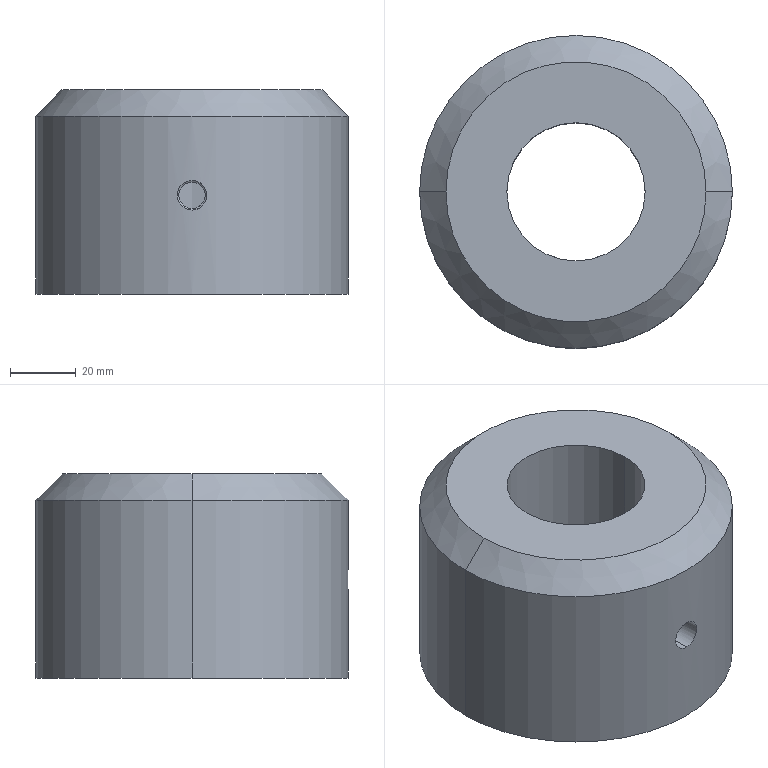Part | SolidWorks | features Chamfer 1, Extrusion 1, HoleWzd 1, ICE 1 | 1 solid | 14 faces | box 95 x 95 x 62 mm | volume 343089 mm3 | cylinder 8 | cone 4 | plane 2 | commonest cylinder face diameters 8 x2 9 x2 42 x2 95 x2
STEP:
#1=CARTESIAN_POINT('',(0.,-37.5,34.5));
#2=VERTEX_POINT('',#1);
#3=CARTESIAN_POINT('',(0.,-37.5,25.5));
#4=VERTEX_POINT('',#3);
#5=CARTESIAN_POINT('',(0.,-37.5,30.));
#6=DIRECTION('',(0.,-1.,0.));
#7=DIRECTION('',(0.,0.,-1.));
#8=AXIS2_PLACEMENT_3D('',#5,#6,#7);
#9=CIRCLE('',#8,4.5);
#10=EDGE_CURVE('',#2,#4,#9,.T.);
#11=ORIENTED_EDGE('',*,*,#10,.F.);
#12=CARTESIAN_POINT('',(0.,-47.5,34.5));
#13=VERTEX_POINT('',#12);
#14=CARTESIAN_POINT('',(0.,-47.5,34.5));
#15=DIRECTION('',(0.,-1.,0.));
#16=VECTOR('',#15,1000.);
#17=LINE('',#14,#16);
#18=EDGE_CURVE('',#2,#13,#17,.T.);
#19=ORIENTED_EDGE('',*,*,#18,.T.);
#20=CARTESIAN_POINT('',(0.,-47.5,25.5));
#21=VERTEX_POINT('',#20);
#22=CARTESIAN_POINT('',(0.,-47.5,25.5));
#23=CARTESIAN_POINT('',(-0.2975,-47.5,25.5));
#24=CARTESIAN_POINT('',(-0.59,-47.497,25.529));
#25=CARTESIAN_POINT('',(-1.165,-47.487,25.644));
#26=CARTESIAN_POINT('',(-1.451,-47.479,25.73));
#27=CARTESIAN_POINT('',(-1.996,-47.459,25.956));
#28=CARTESIAN_POINT('',(-2.255,-47.447,26.094));
#29=CARTESIAN_POINT('',(-2.744,-47.421,26.421));
#30=CARTESIAN_POINT('',(-2.975,-47.407,26.611));
#31=CARTESIAN_POINT('',(-3.39,-47.379,27.026));
#32=CARTESIAN_POINT('',(-3.576,-47.365,27.253));
#33=CARTESIAN_POINT('',(-3.905,-47.339,27.745));
#34=CARTESIAN_POINT('',(-4.045,-47.328,28.006));
#35=CARTESIAN_POINT('',(-4.269,-47.308,28.548));
#36=CARTESIAN_POINT('',(-4.356,-47.3,28.832));
#37=CARTESIAN_POINT('',(-4.471,-47.289,29.413));
#38=CARTESIAN_POINT('',(-4.5,-47.286,29.705));
#39=CARTESIAN_POINT('',(-4.5,-47.286,30.292));
#40=CARTESIAN_POINT('',(-4.471,-47.289,30.59));
#41=CARTESIAN_POINT('',(-4.356,-47.3,31.168));
#42=CARTESIAN_POINT('',(-4.271,-47.308,31.448));
#43=CARTESIAN_POINT('',(-4.045,-47.328,31.993));
#44=CARTESIAN_POINT('',(-3.904,-47.34,32.257));
#45=CARTESIAN_POINT('',(-3.579,-47.365,32.744));
#46=CARTESIAN_POINT('',(-3.393,-47.379,32.971));
#47=CARTESIAN_POINT('',(-2.972,-47.407,33.392));
#48=CARTESIAN_POINT('',(-2.745,-47.421,33.578));
#49=CARTESIAN_POINT('',(-2.258,-47.447,33.904));
#50=CARTESIAN_POINT('',(-1.995,-47.459,34.044));
#51=CARTESIAN_POINT('',(-1.45,-47.479,34.27));
#52=CARTESIAN_POINT('',(-1.169,-47.486,34.355));
#53=CARTESIAN_POINT('',(-0.5922,-47.497,34.471));
#54=CARTESIAN_POINT('',(-0.2938,-47.5,34.5));
#55=CARTESIAN_POINT('',(0.,-47.5,34.5));
#56=B_SPLINE_CURVE_WITH_KNOTS('',3,(#22,#23,#24,#25,#26,#27,#28,#29,#30,#31,#32,#33,#34,#35,#36,#37,#38,#39,#40,#41,#42,#43,#44,#45,#46,#47,#48,#49,#50,#51,#52,#53,#54,#55),.UNSPECIFIED.,.F.,.F.,(4,2,2,2,2,2,2,2,2,2,2,2,2,2,2,2,4),(0.,0.0008798,0.00176,0.002639,0.003519,0.004399,0.005279,0.006159,0.007038,0.007918,0.008798,0.009678,0.01056,0.01144,0.01232,0.0132,0.01408),.UNSPECIFIED.);
#57=EDGE_CURVE('',#21,#13,#56,.T.);
#58=ORIENTED_EDGE('',*,*,#57,.F.);
#59=CARTESIAN_POINT('',(0.,-47.5,25.5));
#60=DIRECTION('',(0.,-1.,0.));
#61=VECTOR('',#60,1000.);
#62=LINE('',#59,#61);
#63=EDGE_CURVE('',#4,#21,#62,.T.);
#64=ORIENTED_EDGE('',*,*,#63,.F.);
#65=EDGE_LOOP('',(#11,#19,#58,#64));
#66=FACE_OUTER_BOUND('',#65,.T.);
#67=CARTESIAN_POINT('',(0.,-47.5,30.));
#68=DIRECTION('',(0.,-1.,0.));
#69=DIRECTION('',(0.,0.,-1.));
#70=AXIS2_PLACEMENT_3D('',#67,#68,#69);
#71=CYLINDRICAL_SURFACE('',#70,4.5);
#72=ADVANCED_FACE('',(#66),#71,.F.);
#73=CARTESIAN_POINT('',(0.,-37.2,34.));
#74=VERTEX_POINT('',#73);
#75=CARTESIAN_POINT('',(0.,-37.2,26.));
#76=VERTEX_POINT('',#75);
#77=CARTESIAN_POINT('',(0.,-37.2,30.));
#78=DIRECTION('',(0.,-1.,0.));
#79=DIRECTION('',(0.,0.,-1.));
#80=AXIS2_PLACEMENT_3D('',#77,#78,#79);
#81=CIRCLE('',#80,4.);
#82=EDGE_CURVE('',#74,#76,#81,.T.);
#83=ORIENTED_EDGE('',*,*,#82,.F.);
#84=CARTESIAN_POINT('',(0.,-37.5,34.5));
#85=DIRECTION('',(0.,-0.515,0.8572));
#86=VECTOR('',#85,1000.);
#87=LINE('',#84,#86);
#88=EDGE_CURVE('',#74,#2,#87,.T.);
#89=ORIENTED_EDGE('',*,*,#88,.T.);
#90=ORIENTED_EDGE('',*,*,#10,.T.);
#91=CARTESIAN_POINT('',(0.,-37.5,25.5));
#92=DIRECTION('',(0.,-0.515,-0.8572));
#93=VECTOR('',#92,1000.);
#94=LINE('',#91,#93);
#95=EDGE_CURVE('',#76,#4,#94,.T.);
#96=ORIENTED_EDGE('',*,*,#95,.F.);
#97=EDGE_LOOP('',(#83,#89,#90,#96));
#98=FACE_OUTER_BOUND('',#97,.T.);
#99=CARTESIAN_POINT('',(0.,-37.5,30.));
#100=DIRECTION('',(0.,-1.,0.));
#101=DIRECTION('',(0.,0.,-1.));
#102=AXIS2_PLACEMENT_3D('',#99,#100,#101);
#103=CONICAL_SURFACE('',#102,4.5,1.03);
#104=ADVANCED_FACE('',(#98),#103,.F.);
#105=ORIENTED_EDGE('',*,*,#82,.T.);
#106=CARTESIAN_POINT('',(0.,-21.,26.));
#107=VERTEX_POINT('',#106);
#108=CARTESIAN_POINT('',(0.,-47.5,26.));
#109=DIRECTION('',(0.,1.,0.));
#110=VECTOR('',#109,1000.);
#111=LINE('',#108,#110);
#112=EDGE_CURVE('',#76,#107,#111,.T.);
#113=ORIENTED_EDGE('',*,*,#112,.T.);
#114=CARTESIAN_POINT('',(0.,-21.,34.));
#115=VERTEX_POINT('',#114);
#116=CARTESIAN_POINT('',(0.,-21.,26.));
#117=CARTESIAN_POINT('',(-0.2613,-21.,26.));
#118=CARTESIAN_POINT('',(-0.5215,-20.995,26.025));
#119=CARTESIAN_POINT('',(-1.039,-20.976,26.128));
#120=CARTESIAN_POINT('',(-1.291,-20.962,26.205));
#121=CARTESIAN_POINT('',(-1.772,-20.926,26.405));
#122=CARTESIAN_POINT('',(-2.006,-20.905,26.529));
#123=CARTESIAN_POINT('',(-2.441,-20.859,26.821));
#124=CARTESIAN_POINT('',(-2.642,-20.834,26.986));
#125=CARTESIAN_POINT('',(-3.011,-20.784,27.354));
#126=CARTESIAN_POINT('',(-3.18,-20.758,27.559));
#127=CARTESIAN_POINT('',(-3.47,-20.712,27.993));
#128=CARTESIAN_POINT('',(-3.593,-20.691,28.222));
#129=CARTESIAN_POINT('',(-3.794,-20.655,28.707));
#130=CARTESIAN_POINT('',(-3.871,-20.64,28.96));
#131=CARTESIAN_POINT('',(-3.974,-20.621,29.472));
#132=CARTESIAN_POINT('',(-4.,-20.616,29.734));
#133=CARTESIAN_POINT('',(-4.,-20.616,30.262));
#134=CARTESIAN_POINT('',(-3.974,-20.621,30.522));
#135=CARTESIAN_POINT('',(-3.873,-20.64,31.035));
#136=CARTESIAN_POINT('',(-3.795,-20.654,31.29));
#137=CARTESIAN_POINT('',(-3.595,-20.69,31.773));
#138=CARTESIAN_POINT('',(-3.473,-20.711,32.003));
#139=CARTESIAN_POINT('',(-3.182,-20.758,32.438));
#140=CARTESIAN_POINT('',(-3.014,-20.783,32.643));
#141=CARTESIAN_POINT('',(-2.647,-20.833,33.011));
#142=CARTESIAN_POINT('',(-2.446,-20.858,33.176));
#143=CARTESIAN_POINT('',(-2.007,-20.905,33.47));
#144=CARTESIAN_POINT('',(-1.777,-20.926,33.593));
#145=CARTESIAN_POINT('',(-1.296,-20.961,33.793));
#146=CARTESIAN_POINT('',(-1.043,-20.976,33.871));
#147=CARTESIAN_POINT('',(-0.5264,-20.995,33.974));
#148=CARTESIAN_POINT('',(-0.2649,-21.,34.));
#149=CARTESIAN_POINT('',(0.,-21.,34.));
#150=B_SPLINE_CURVE_WITH_KNOTS('',3,(#116,#117,#118,#119,#120,#121,#122,#123,#124,#125,#126,#127,#128,#129,#130,#131,#132,#133,#134,#135,#136,#137,#138,#139,#140,#141,#142,#143,#144,#145,#146,#147,#148,#149),.UNSPECIFIED.,.F.,.F.,(4,2,2,2,2,2,2,2,2,2,2,2,2,2,2,2,4),(0.01253,0.01332,0.0141,0.01488,0.01567,0.01645,0.01723,0.01802,0.0188,0.01958,0.02037,0.02115,0.02193,0.02272,0.0235,0.02428,0.02507),.UNSPECIFIED.);
#151=EDGE_CURVE('',#107,#115,#150,.T.);
#152=ORIENTED_EDGE('',*,*,#151,.T.);
#153=CARTESIAN_POINT('',(0.,-47.5,34.));
#154=DIRECTION('',(0.,1.,0.));
#155=VECTOR('',#154,1000.);
#156=LINE('',#153,#155);
#157=EDGE_CURVE('',#74,#115,#156,.T.);
#158=ORIENTED_EDGE('',*,*,#157,.F.);
#159=EDGE_LOOP('',(#105,#113,#152,#158));
#160=FACE_OUTER_BOUND('',#159,.T.);
#161=CARTESIAN_POINT('',(0.,-47.5,30.));
#162=DIRECTION('',(0.,1.,0.));
#163=DIRECTION('',(0.,0.,1.));
#164=AXIS2_PLACEMENT_3D('',#161,#162,#163);
#165=CYLINDRICAL_SURFACE('',#164,4.);
#166=ADVANCED_FACE('',(#160),#165,.F.);
#167=CARTESIAN_POINT('',(39.5,0.,62.));
#168=VERTEX_POINT('',#167);
#169=CARTESIAN_POINT('',(-39.5,0.,62.));
#170=VERTEX_POINT('',#169);
#171=CARTESIAN_POINT('',(0.,0.,62.));
#172=DIRECTION('',(0.,0.,1.));
#173=DIRECTION('',(1.,0.,0.));
#174=AXIS2_PLACEMENT_3D('',#171,#172,#173);
#175=CIRCLE('',#174,39.5);
#176=EDGE_CURVE('',#168,#170,#175,.T.);
#177=ORIENTED_EDGE('',*,*,#176,.F.);
#178=CARTESIAN_POINT('',(47.5,0.,54.));
#179=VERTEX_POINT('',#178);
#180=CARTESIAN_POINT('',(39.5,0.,62.));
#181=DIRECTION('',(0.7071,0.,-0.7071));
#182=VECTOR('',#181,1000.);
#183=LINE('',#180,#182);
#184=EDGE_CURVE('',#168,#179,#183,.T.);
#185=ORIENTED_EDGE('',*,*,#184,.T.);
#186=CARTESIAN_POINT('',(-47.5,0.,54.));
#187=VERTEX_POINT('',#186);
#188=CARTESIAN_POINT('',(0.,0.,54.));
#189=DIRECTION('',(0.,0.,-1.));
#190=DIRECTION('',(1.,0.,0.));
#191=AXIS2_PLACEMENT_3D('',#188,#189,#190);
#192=CIRCLE('',#191,47.5);
#193=EDGE_CURVE('',#187,#179,#192,.T.);
#194=ORIENTED_EDGE('',*,*,#193,.F.);
#195=CARTESIAN_POINT('',(-39.5,0.,62.));
#196=DIRECTION('',(-0.7071,0.,-0.7071));
#197=VECTOR('',#196,1000.);
#198=LINE('',#195,#197);
#199=EDGE_CURVE('',#170,#187,#198,.T.);
#200=ORIENTED_EDGE('',*,*,#199,.F.);
#201=EDGE_LOOP('',(#177,#185,#194,#200));
#202=FACE_OUTER_BOUND('',#201,.T.);
#203=CARTESIAN_POINT('',(0.,0.,62.));
#204=DIRECTION('',(0.,0.,-1.));
#205=DIRECTION('',(-1.,0.,0.));
#206=AXIS2_PLACEMENT_3D('',#203,#204,#205);
#207=CONICAL_SURFACE('',#206,39.5,0.7854);
#208=ADVANCED_FACE('',(#202),#207,.T.);
#209=CARTESIAN_POINT('',(0.,-21.,34.));
#210=CARTESIAN_POINT('',(0.2649,-21.,34.));
#211=CARTESIAN_POINT('',(0.5253,-20.995,33.974));
#212=CARTESIAN_POINT('',(1.037,-20.976,33.872));
#213=CARTESIAN_POINT('',(1.292,-20.962,33.795));
#214=CARTESIAN_POINT('',(1.776,-20.926,33.594));
#215=CARTESIAN_POINT('',(2.006,-20.905,33.471));
#216=CARTESIAN_POINT('',(2.44,-20.859,33.18));
#217=CARTESIAN_POINT('',(2.645,-20.834,33.012));
#218=CARTESIAN_POINT('',(3.013,-20.784,32.644));
#219=CARTESIAN_POINT('',(3.178,-20.759,32.443));
#220=CARTESIAN_POINT('',(3.471,-20.712,32.006));
#221=CARTESIAN_POINT('',(3.595,-20.69,31.774));
#222=CARTESIAN_POINT('',(3.794,-20.655,31.293));
#223=CARTESIAN_POINT('',(3.871,-20.64,31.04));
#224=CARTESIAN_POINT('',(3.974,-20.621,30.523));
#225=CARTESIAN_POINT('',(4.,-20.616,30.263));
#226=CARTESIAN_POINT('',(4.,-20.616,29.74));
#227=CARTESIAN_POINT('',(3.974,-20.621,29.474));
#228=CARTESIAN_POINT('',(3.871,-20.64,28.961));
#229=CARTESIAN_POINT('',(3.796,-20.654,28.711));
#230=CARTESIAN_POINT('',(3.595,-20.69,28.226));
#231=CARTESIAN_POINT('',(3.47,-20.712,27.993));
#232=CARTESIAN_POINT('',(3.18,-20.758,27.56));
#233=CARTESIAN_POINT('',(3.014,-20.783,27.357));
#234=CARTESIAN_POINT('',(2.642,-20.834,26.985));
#235=CARTESIAN_POINT('',(2.441,-20.859,26.82));
#236=CARTESIAN_POINT('',(2.008,-20.905,26.531));
#237=CARTESIAN_POINT('',(1.774,-20.926,26.405));
#238=CARTESIAN_POINT('',(1.29,-20.962,26.205));
#239=CARTESIAN_POINT('',(1.041,-20.976,26.129));
#240=CARTESIAN_POINT('',(0.5269,-20.995,26.026));
#241=CARTESIAN_POINT('',(0.2614,-21.,26.));
#242=CARTESIAN_POINT('',(0.,-21.,26.));
#243=B_SPLINE_CURVE_WITH_KNOTS('',3,(#209,#210,#211,#212,#213,#214,#215,#216,#217,#218,#219,#220,#221,#222,#223,#224,#225,#226,#227,#228,#229,#230,#231,#232,#233,#234,#235,#236,#237,#238,#239,#240,#241,#242),.UNSPECIFIED.,.F.,.F.,(4,2,2,2,2,2,2,2,2,2,2,2,2,2,2,2,4),(0.,0.0007834,0.001567,0.00235,0.003134,0.003917,0.0047,0.005484,0.006267,0.007051,0.007834,0.008617,0.009401,0.01018,0.01097,0.01175,0.01253),.UNSPECIFIED.);
#244=EDGE_CURVE('',#115,#107,#243,.T.);
#245=ORIENTED_EDGE('',*,*,#244,.F.);
#246=ORIENTED_EDGE('',*,*,#151,.F.);
#247=EDGE_LOOP('',(#245,#246));
#248=FACE_BOUND('',#247,.T.);
#249=CARTESIAN_POINT('',(-21.,0.,62.));
#250=VERTEX_POINT('',#249);
#251=CARTESIAN_POINT('',(21.,0.,62.));
#252=VERTEX_POINT('',#251);
#253=CARTESIAN_POINT('',(0.,0.,62.));
#254=DIRECTION('',(0.,0.,1.));
#255=DIRECTION('',(1.,0.,0.));
#256=AXIS2_PLACEMENT_3D('',#253,#254,#255);
#257=CIRCLE('',#256,21.);
#258=EDGE_CURVE('',#250,#252,#257,.T.);
#259=ORIENTED_EDGE('',*,*,#258,.T.);
#260=CARTESIAN_POINT('',(21.,0.,0.));
#261=VERTEX_POINT('',#260);
#262=CARTESIAN_POINT('',(21.,0.,62.));
#263=DIRECTION('',(0.,0.,-1.));
#264=VECTOR('',#263,1000.);
#265=LINE('',#262,#264);
#266=EDGE_CURVE('',#252,#261,#265,.T.);
#267=ORIENTED_EDGE('',*,*,#266,.T.);
#268=CARTESIAN_POINT('',(-21.,0.,0.));
#269=VERTEX_POINT('',#268);
#270=CARTESIAN_POINT('',(0.,0.,0.));
#271=DIRECTION('',(0.,0.,1.));
#272=DIRECTION('',(1.,0.,0.));
#273=AXIS2_PLACEMENT_3D('',#270,#271,#272);
#274=CIRCLE('',#273,21.);
#275=EDGE_CURVE('',#269,#261,#274,.T.);
#276=ORIENTED_EDGE('',*,*,#275,.F.);
#277=CARTESIAN_POINT('',(-21.,0.,62.));
#278=DIRECTION('',(0.,0.,-1.));
#279=VECTOR('',#278,1000.);
#280=LINE('',#277,#279);
#281=EDGE_CURVE('',#250,#269,#280,.T.);
#282=ORIENTED_EDGE('',*,*,#281,.F.);
#283=EDGE_LOOP('',(#259,#267,#276,#282));
#284=FACE_OUTER_BOUND('',#283,.T.);
#285=CARTESIAN_POINT('',(0.,0.,62.));
#286=DIRECTION('',(0.,0.,-1.));
#287=DIRECTION('',(-1.,0.,0.));
#288=AXIS2_PLACEMENT_3D('',#285,#286,#287);
#289=CYLINDRICAL_SURFACE('',#288,21.);
#290=ADVANCED_FACE('',(#248,#284),#289,.F.);
#291=ORIENTED_EDGE('',*,*,#193,.T.);
#292=CARTESIAN_POINT('',(47.5,0.,0.));
#293=VERTEX_POINT('',#292);
#294=CARTESIAN_POINT('',(47.5,0.,62.));
#295=DIRECTION('',(0.,0.,-1.));
#296=VECTOR('',#295,1000.);
#297=LINE('',#294,#296);
#298=EDGE_CURVE('',#179,#293,#297,.T.);
#299=ORIENTED_EDGE('',*,*,#298,.T.);
#300=CARTESIAN_POINT('',(-47.5,0.,0.));
#301=VERTEX_POINT('',#300);
#302=CARTESIAN_POINT('',(0.,0.,0.));
#303=DIRECTION('',(0.,0.,1.));
#304=DIRECTION('',(1.,0.,0.));
#305=AXIS2_PLACEMENT_3D('',#302,#303,#304);
#306=CIRCLE('',#305,47.5);
#307=EDGE_CURVE('',#293,#301,#306,.T.);
#308=ORIENTED_EDGE('',*,*,#307,.T.);
#309=CARTESIAN_POINT('',(-47.5,0.,62.));
#310=DIRECTION('',(0.,0.,-1.));
#311=VECTOR('',#310,1000.);
#312=LINE('',#309,#311);
#313=EDGE_CURVE('',#187,#301,#312,.T.);
#314=ORIENTED_EDGE('',*,*,#313,.F.);
#315=EDGE_LOOP('',(#291,#299,#308,#314));
#316=FACE_OUTER_BOUND('',#315,.T.);
#317=CARTESIAN_POINT('',(0.,0.,62.));
#318=DIRECTION('',(0.,0.,-1.));
#319=DIRECTION('',(-1.,0.,0.));
#320=AXIS2_PLACEMENT_3D('',#317,#318,#319);
#321=CYLINDRICAL_SURFACE('',#320,47.5);
#322=ADVANCED_FACE('',(#316),#321,.T.);
#323=CARTESIAN_POINT('',(0.,0.,62.));
#324=DIRECTION('',(0.,0.,1.));
#325=DIRECTION('',(1.,0.,0.));
#326=AXIS2_PLACEMENT_3D('',#323,#324,#325);
#327=CIRCLE('',#326,39.5);
#328=EDGE_CURVE('',#170,#168,#327,.T.);
#329=ORIENTED_EDGE('',*,*,#328,.T.);
#330=ORIENTED_EDGE('',*,*,#176,.T.);
#331=EDGE_LOOP('',(#329,#330));
#332=FACE_OUTER_BOUND('',#331,.T.);
#333=ORIENTED_EDGE('',*,*,#258,.F.);
#334=CARTESIAN_POINT('',(0.,0.,62.));
#335=DIRECTION('',(0.,0.,1.));
#336=DIRECTION('',(1.,0.,0.));
#337=AXIS2_PLACEMENT_3D('',#334,#335,#336);
#338=CIRCLE('',#337,21.);
#339=EDGE_CURVE('',#252,#250,#338,.T.);
#340=ORIENTED_EDGE('',*,*,#339,.F.);
#341=EDGE_LOOP('',(#333,#340));
#342=FACE_BOUND('',#341,.T.);
#343=CARTESIAN_POINT('',(0.,0.,62.));
#344=DIRECTION('',(0.,0.,1.));
#345=DIRECTION('',(1.,0.,0.));
#346=AXIS2_PLACEMENT_3D('',#343,#344,#345);
#347=PLANE('',#346);
#348=ADVANCED_FACE('',(#332,#342),#347,.T.);
#349=CARTESIAN_POINT('',(0.,0.,0.));
#350=DIRECTION('',(0.,0.,1.));
#351=DIRECTION('',(1.,0.,0.));
#352=AXIS2_PLACEMENT_3D('',#349,#350,#351);
#353=CIRCLE('',#352,47.5);
#354=EDGE_CURVE('',#301,#293,#353,.T.);
#355=ORIENTED_EDGE('',*,*,#354,.F.);
#356=ORIENTED_EDGE('',*,*,#307,.F.);
#357=EDGE_LOOP('',(#355,#356));
#358=FACE_OUTER_BOUND('',#357,.T.);
#359=ORIENTED_EDGE('',*,*,#275,.T.);
#360=CARTESIAN_POINT('',(0.,0.,0.));
#361=DIRECTION('',(0.,0.,1.));
#362=DIRECTION('',(1.,0.,0.));
#363=AXIS2_PLACEMENT_3D('',#360,#361,#362);
#364=CIRCLE('',#363,21.);
#365=EDGE_CURVE('',#261,#269,#364,.T.);
#366=ORIENTED_EDGE('',*,*,#365,.T.);
#367=EDGE_LOOP('',(#359,#366));
#368=FACE_BOUND('',#367,.T.);
#369=CARTESIAN_POINT('',(0.,0.,0.));
#370=DIRECTION('',(0.,0.,1.));
#371=DIRECTION('',(1.,0.,0.));
#372=AXIS2_PLACEMENT_3D('',#369,#370,#371);
#373=PLANE('',#372);
#374=ADVANCED_FACE('',(#358,#368),#373,.F.);
#375=ORIENTED_EDGE('',*,*,#298,.F.);
#376=CARTESIAN_POINT('',(0.,0.,54.));
#377=DIRECTION('',(0.,0.,-1.));
#378=DIRECTION('',(1.,0.,0.));
#379=AXIS2_PLACEMENT_3D('',#376,#377,#378);
#380=CIRCLE('',#379,47.5);
#381=EDGE_CURVE('',#179,#187,#380,.T.);
#382=ORIENTED_EDGE('',*,*,#381,.T.);
#383=ORIENTED_EDGE('',*,*,#313,.T.);
#384=ORIENTED_EDGE('',*,*,#354,.T.);
#385=EDGE_LOOP('',(#375,#382,#383,#384));
#386=FACE_OUTER_BOUND('',#385,.T.);
#387=ORIENTED_EDGE('',*,*,#57,.T.);
#388=CARTESIAN_POINT('',(0.,-47.5,34.5));
#389=CARTESIAN_POINT('',(0.2937,-47.5,34.5));
#390=CARTESIAN_POINT('',(0.5857,-47.497,34.472));
#391=CARTESIAN_POINT('',(1.166,-47.487,34.356));
#392=CARTESIAN_POINT('',(1.45,-47.479,34.27));
#393=CARTESIAN_POINT('',(1.992,-47.459,34.046));
#394=CARTESIAN_POINT('',(2.254,-47.447,33.906));
#395=CARTESIAN_POINT('',(2.746,-47.421,33.578));
#396=CARTESIAN_POINT('',(2.972,-47.407,33.391));
#397=CARTESIAN_POINT('',(3.387,-47.38,32.977));
#398=CARTESIAN_POINT('',(3.577,-47.365,32.746));
#399=CARTESIAN_POINT('',(3.904,-47.34,32.257));
#400=CARTESIAN_POINT('',(4.043,-47.328,31.999));
#401=CARTESIAN_POINT('',(4.269,-47.308,31.454));
#402=CARTESIAN_POINT('',(4.356,-47.3,31.168));
#403=CARTESIAN_POINT('',(4.47,-47.289,30.593));
#404=CARTESIAN_POINT('',(4.5,-47.286,30.301));
#405=CARTESIAN_POINT('',(4.5,-47.286,29.706));
#406=CARTESIAN_POINT('',(4.471,-47.289,29.413));
#407=CARTESIAN_POINT('',(4.357,-47.3,28.838));
#408=CARTESIAN_POINT('',(4.271,-47.308,28.552));
#409=CARTESIAN_POINT('',(4.045,-47.328,28.007));
#410=CARTESIAN_POINT('',(3.907,-47.339,27.749));
#411=CARTESIAN_POINT('',(3.581,-47.365,27.259));
#412=CARTESIAN_POINT('',(3.392,-47.379,27.028));
#413=CARTESIAN_POINT('',(2.977,-47.407,26.613));
#414=CARTESIAN_POINT('',(2.751,-47.421,26.426));
#415=CARTESIAN_POINT('',(2.259,-47.447,26.097));
#416=CARTESIAN_POINT('',(1.998,-47.459,25.957));
#417=CARTESIAN_POINT('',(1.456,-47.478,25.732));
#418=CARTESIAN_POINT('',(1.174,-47.486,25.646));
#419=CARTESIAN_POINT('',(0.5916,-47.497,25.529));
#420=CARTESIAN_POINT('',(0.2974,-47.5,25.5));
#421=CARTESIAN_POINT('',(0.,-47.5,25.5));
#422=B_SPLINE_CURVE_WITH_KNOTS('',3,(#388,#389,#390,#391,#392,#393,#394,#395,#396,#397,#398,#399,#400,#401,#402,#403,#404,#405,#406,#407,#408,#409,#410,#411,#412,#413,#414,#415,#416,#417,#418,#419,#420,#421),.UNSPECIFIED.,.F.,.F.,(4,2,2,2,2,2,2,2,2,2,2,2,2,2,2,2,4),(0.01408,0.01496,0.01584,0.01672,0.0176,0.01847,0.01935,0.02023,0.02111,0.02199,0.02287,0.02375,0.02463,0.02551,0.02639,0.02727,0.02815),.UNSPECIFIED.);
#423=EDGE_CURVE('',#13,#21,#422,.T.);
#424=ORIENTED_EDGE('',*,*,#423,.T.);
#425=EDGE_LOOP('',(#387,#424));
#426=FACE_BOUND('',#425,.T.);
#427=CARTESIAN_POINT('',(0.,0.,62.));
#428=DIRECTION('',(0.,0.,-1.));
#429=DIRECTION('',(-1.,0.,0.));
#430=AXIS2_PLACEMENT_3D('',#427,#428,#429);
#431=CYLINDRICAL_SURFACE('',#430,47.5);
#432=ADVANCED_FACE('',(#386,#426),#431,.T.);
#433=ORIENTED_EDGE('',*,*,#266,.F.);
#434=ORIENTED_EDGE('',*,*,#339,.T.);
#435=ORIENTED_EDGE('',*,*,#281,.T.);
#436=ORIENTED_EDGE('',*,*,#365,.F.);
#437=EDGE_LOOP('',(#433,#434,#435,#436));
#438=FACE_OUTER_BOUND('',#437,.T.);
#439=CARTESIAN_POINT('',(0.,0.,62.));
#440=DIRECTION('',(0.,0.,-1.));
#441=DIRECTION('',(-1.,0.,0.));
#442=AXIS2_PLACEMENT_3D('',#439,#440,#441);
#443=CYLINDRICAL_SURFACE('',#442,21.);
#444=ADVANCED_FACE('',(#438),#443,.F.);
#445=ORIENTED_EDGE('',*,*,#184,.F.);
#446=ORIENTED_EDGE('',*,*,#328,.F.);
#447=ORIENTED_EDGE('',*,*,#199,.T.);
#448=ORIENTED_EDGE('',*,*,#381,.F.);
#449=EDGE_LOOP('',(#445,#446,#447,#448));
#450=FACE_OUTER_BOUND('',#449,.T.);
#451=CARTESIAN_POINT('',(0.,0.,62.));
#452=DIRECTION('',(0.,0.,-1.));
#453=DIRECTION('',(-1.,0.,0.));
#454=AXIS2_PLACEMENT_3D('',#451,#452,#453);
#455=CONICAL_SURFACE('',#454,39.5,0.7854);
#456=ADVANCED_FACE('',(#450),#455,.T.);
#457=ORIENTED_EDGE('',*,*,#112,.F.);
#458=CARTESIAN_POINT('',(0.,-37.2,30.));
#459=DIRECTION('',(0.,-1.,0.));
#460=DIRECTION('',(0.,0.,-1.));
#461=AXIS2_PLACEMENT_3D('',#458,#459,#460);
#462=CIRCLE('',#461,4.);
#463=EDGE_CURVE('',#76,#74,#462,.T.);
#464=ORIENTED_EDGE('',*,*,#463,.T.);
#465=ORIENTED_EDGE('',*,*,#157,.T.);
#466=ORIENTED_EDGE('',*,*,#244,.T.);
#467=EDGE_LOOP('',(#457,#464,#465,#466));
#468=FACE_OUTER_BOUND('',#467,.T.);
#469=CARTESIAN_POINT('',(0.,-47.5,30.));
#470=DIRECTION('',(0.,1.,0.));
#471=DIRECTION('',(0.,0.,1.));
#472=AXIS2_PLACEMENT_3D('',#469,#470,#471);
#473=CYLINDRICAL_SURFACE('',#472,4.);
#474=ADVANCED_FACE('',(#468),#473,.F.);
#475=ORIENTED_EDGE('',*,*,#88,.F.);
#476=ORIENTED_EDGE('',*,*,#463,.F.);
#477=ORIENTED_EDGE('',*,*,#95,.T.);
#478=CARTESIAN_POINT('',(0.,-37.5,30.));
#479=DIRECTION('',(0.,-1.,0.));
#480=DIRECTION('',(0.,0.,-1.));
#481=AXIS2_PLACEMENT_3D('',#478,#479,#480);
#482=CIRCLE('',#481,4.5);
#483=EDGE_CURVE('',#4,#2,#482,.T.);
#484=ORIENTED_EDGE('',*,*,#483,.T.);
#485=EDGE_LOOP('',(#475,#476,#477,#484));
#486=FACE_OUTER_BOUND('',#485,.T.);
#487=CARTESIAN_POINT('',(0.,-37.5,30.));
#488=DIRECTION('',(0.,-1.,0.));
#489=DIRECTION('',(0.,0.,-1.));
#490=AXIS2_PLACEMENT_3D('',#487,#488,#489);
#491=CONICAL_SURFACE('',#490,4.5,1.03);
#492=ADVANCED_FACE('',(#486),#491,.F.);
#493=ORIENTED_EDGE('',*,*,#18,.F.);
#494=ORIENTED_EDGE('',*,*,#483,.F.);
#495=ORIENTED_EDGE('',*,*,#63,.T.);
#496=ORIENTED_EDGE('',*,*,#423,.F.);
#497=EDGE_LOOP('',(#493,#494,#495,#496));
#498=FACE_OUTER_BOUND('',#497,.T.);
#499=CARTESIAN_POINT('',(0.,-47.5,30.));
#500=DIRECTION('',(0.,-1.,0.));
#501=DIRECTION('',(0.,0.,-1.));
#502=AXIS2_PLACEMENT_3D('',#499,#500,#501);
#503=CYLINDRICAL_SURFACE('',#502,4.5);
#504=ADVANCED_FACE('',(#498),#503,.F.);
#505=CLOSED_SHELL('',(#72,#104,#166,#208,#290,#322,#348,#374,#432,#444,#456,#474,#492,#504));
#506=MANIFOLD_SOLID_BREP('',#505);
#507=CARTESIAN_POINT('',(0.,0.,0.));
#508=DIRECTION('',(0.,0.,1.));
#509=DIRECTION('',(1.,0.,0.));
#510=AXIS2_PLACEMENT_3D('',#507,#508,#509);
#511=(LENGTH_UNIT()NAMED_UNIT(*)SI_UNIT(.MILLI.,.METRE.));
#512=UNCERTAINTY_MEASURE_WITH_UNIT(LENGTH_MEASURE(0.00001),#511,'','');
#513=(NAMED_UNIT(*)PLANE_ANGLE_UNIT()SI_UNIT($,.RADIAN.));
#514=(NAMED_UNIT(*)SI_UNIT($,.STERADIAN.)SOLID_ANGLE_UNIT());
#515=(GEOMETRIC_REPRESENTATION_CONTEXT(3)GLOBAL_UNCERTAINTY_ASSIGNED_CONTEXT((#512))GLOBAL_UNIT_ASSIGNED_CONTEXT((#511,#513,#514))REPRESENTATION_CONTEXT('',''));
#516=ADVANCED_BREP_SHAPE_REPRESENTATION('',(#506,#510),#515);